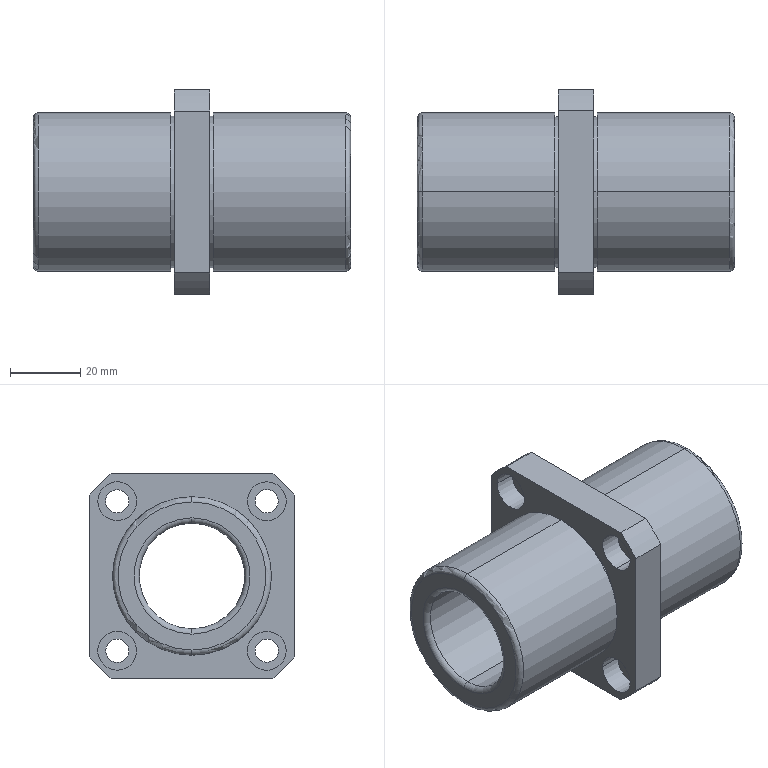Part | SolidWorks | features ICE 3, CirPattern 1, Fillet 1, Revolution 1 | 1 solid | 52 faces | box 90 x 58 x 58 mm | volume 93231 mm3 | cylinder 30 | plane 14 | torus 8 | commonest cylinder face diameters 6.6 x8 11 x8 43 x4 45 x4 74 x4 30 x2
STEP:
#1=CARTESIAN_POINT('',(-40.,0.,21.));
#2=VERTEX_POINT('',#1);
#3=CARTESIAN_POINT('',(-40.,0.,-21.));
#4=VERTEX_POINT('',#3);
#5=CARTESIAN_POINT('',(-40.,0.,0.));
#6=DIRECTION('',(-1.,0.,0.));
#7=DIRECTION('',(0.,0.,-1.));
#8=AXIS2_PLACEMENT_3D('',#5,#6,#7);
#9=CIRCLE('',#8,21.);
#10=EDGE_CURVE('',#2,#4,#9,.T.);
#11=ORIENTED_EDGE('',*,*,#10,.F.);
#12=CARTESIAN_POINT('',(-38.5,0.,22.5));
#13=VERTEX_POINT('',#12);
#14=CARTESIAN_POINT('',(-38.5,0.,21.));
#15=DIRECTION('',(0.,1.,0.));
#16=DIRECTION('',(0.,0.,1.));
#17=AXIS2_PLACEMENT_3D('',#14,#15,#16);
#18=CIRCLE('',#17,1.5);
#19=EDGE_CURVE('',#2,#13,#18,.T.);
#20=ORIENTED_EDGE('',*,*,#19,.T.);
#21=CARTESIAN_POINT('',(-38.5,0.,-22.5));
#22=VERTEX_POINT('',#21);
#23=CARTESIAN_POINT('',(-38.5,0.,0.));
#24=DIRECTION('',(1.,0.,0.));
#25=DIRECTION('',(0.,0.,-1.));
#26=AXIS2_PLACEMENT_3D('',#23,#24,#25);
#27=CIRCLE('',#26,22.5);
#28=EDGE_CURVE('',#22,#13,#27,.T.);
#29=ORIENTED_EDGE('',*,*,#28,.F.);
#30=CARTESIAN_POINT('',(-38.5,0.,-21.));
#31=DIRECTION('',(0.,-1.,0.));
#32=DIRECTION('',(0.,0.,-1.));
#33=AXIS2_PLACEMENT_3D('',#30,#31,#32);
#34=CIRCLE('',#33,1.5);
#35=EDGE_CURVE('',#4,#22,#34,.T.);
#36=ORIENTED_EDGE('',*,*,#35,.F.);
#37=EDGE_LOOP('',(#11,#20,#29,#36));
#38=FACE_OUTER_BOUND('',#37,.T.);
#39=CARTESIAN_POINT('',(-38.5,0.,0.));
#40=DIRECTION('',(1.,0.,0.));
#41=DIRECTION('',(0.,0.,-1.));
#42=AXIS2_PLACEMENT_3D('',#39,#40,#41);
#43=TOROIDAL_SURFACE('',#42,21.,1.5);
#44=ADVANCED_FACE('',(#38),#43,.T.);
#45=CARTESIAN_POINT('',(50.,0.,-21.));
#46=VERTEX_POINT('',#45);
#47=CARTESIAN_POINT('',(50.,0.,21.));
#48=VERTEX_POINT('',#47);
#49=CARTESIAN_POINT('',(50.,0.,0.));
#50=DIRECTION('',(1.,0.,0.));
#51=DIRECTION('',(0.,0.,1.));
#52=AXIS2_PLACEMENT_3D('',#49,#50,#51);
#53=CIRCLE('',#52,21.);
#54=EDGE_CURVE('',#46,#48,#53,.T.);
#55=ORIENTED_EDGE('',*,*,#54,.F.);
#56=CARTESIAN_POINT('',(48.5,0.,-22.5));
#57=VERTEX_POINT('',#56);
#58=CARTESIAN_POINT('',(48.5,0.,-21.));
#59=DIRECTION('',(0.,1.,0.));
#60=DIRECTION('',(0.,0.,1.));
#61=AXIS2_PLACEMENT_3D('',#58,#59,#60);
#62=CIRCLE('',#61,1.5);
#63=EDGE_CURVE('',#46,#57,#62,.T.);
#64=ORIENTED_EDGE('',*,*,#63,.T.);
#65=CARTESIAN_POINT('',(48.5,0.,22.5));
#66=VERTEX_POINT('',#65);
#67=CARTESIAN_POINT('',(48.5,0.,0.));
#68=DIRECTION('',(-1.,0.,0.));
#69=DIRECTION('',(0.,0.,1.));
#70=AXIS2_PLACEMENT_3D('',#67,#68,#69);
#71=CIRCLE('',#70,22.5);
#72=EDGE_CURVE('',#66,#57,#71,.T.);
#73=ORIENTED_EDGE('',*,*,#72,.F.);
#74=CARTESIAN_POINT('',(48.5,0.,21.));
#75=DIRECTION('',(0.,-1.,0.));
#76=DIRECTION('',(0.,0.,-1.));
#77=AXIS2_PLACEMENT_3D('',#74,#75,#76);
#78=CIRCLE('',#77,1.5);
#79=EDGE_CURVE('',#48,#66,#78,.T.);
#80=ORIENTED_EDGE('',*,*,#79,.F.);
#81=EDGE_LOOP('',(#55,#64,#73,#80));
#82=FACE_OUTER_BOUND('',#81,.T.);
#83=CARTESIAN_POINT('',(48.5,0.,0.));
#84=DIRECTION('',(-1.,0.,0.));
#85=DIRECTION('',(0.,0.,1.));
#86=AXIS2_PLACEMENT_3D('',#83,#84,#85);
#87=TOROIDAL_SURFACE('',#86,21.,1.5);
#88=ADVANCED_FACE('',(#82),#87,.T.);
#89=CARTESIAN_POINT('',(48.5,0.,-15.));
#90=VERTEX_POINT('',#89);
#91=CARTESIAN_POINT('',(48.5,0.,15.));
#92=VERTEX_POINT('',#91);
#93=CARTESIAN_POINT('',(48.5,0.,0.));
#94=DIRECTION('',(1.,0.,0.));
#95=DIRECTION('',(0.,0.,1.));
#96=AXIS2_PLACEMENT_3D('',#93,#94,#95);
#97=CIRCLE('',#96,15.);
#98=EDGE_CURVE('',#90,#92,#97,.T.);
#99=ORIENTED_EDGE('',*,*,#98,.F.);
#100=CARTESIAN_POINT('',(50.,0.,-16.5));
#101=VERTEX_POINT('',#100);
#102=CARTESIAN_POINT('',(48.5,0.,-16.5));
#103=DIRECTION('',(0.,1.,0.));
#104=DIRECTION('',(0.,0.,1.));
#105=AXIS2_PLACEMENT_3D('',#102,#103,#104);
#106=CIRCLE('',#105,1.5);
#107=EDGE_CURVE('',#90,#101,#106,.T.);
#108=ORIENTED_EDGE('',*,*,#107,.T.);
#109=CARTESIAN_POINT('',(50.,0.,16.5));
#110=VERTEX_POINT('',#109);
#111=CARTESIAN_POINT('',(50.,0.,0.));
#112=DIRECTION('',(-1.,0.,0.));
#113=DIRECTION('',(0.,0.,1.));
#114=AXIS2_PLACEMENT_3D('',#111,#112,#113);
#115=CIRCLE('',#114,16.5);
#116=EDGE_CURVE('',#110,#101,#115,.T.);
#117=ORIENTED_EDGE('',*,*,#116,.F.);
#118=CARTESIAN_POINT('',(48.5,0.,16.5));
#119=DIRECTION('',(0.,-1.,0.));
#120=DIRECTION('',(0.,0.,-1.));
#121=AXIS2_PLACEMENT_3D('',#118,#119,#120);
#122=CIRCLE('',#121,1.5);
#123=EDGE_CURVE('',#92,#110,#122,.T.);
#124=ORIENTED_EDGE('',*,*,#123,.F.);
#125=EDGE_LOOP('',(#99,#108,#117,#124));
#126=FACE_OUTER_BOUND('',#125,.T.);
#127=CARTESIAN_POINT('',(48.5,0.,0.));
#128=DIRECTION('',(-1.,0.,0.));
#129=DIRECTION('',(0.,0.,1.));
#130=AXIS2_PLACEMENT_3D('',#127,#128,#129);
#131=TOROIDAL_SURFACE('',#130,16.5,1.5);
#132=ADVANCED_FACE('',(#126),#131,.T.);
#133=CARTESIAN_POINT('',(-38.5,0.,15.));
#134=VERTEX_POINT('',#133);
#135=CARTESIAN_POINT('',(-38.5,0.,-15.));
#136=VERTEX_POINT('',#135);
#137=CARTESIAN_POINT('',(-38.5,0.,0.));
#138=DIRECTION('',(-1.,0.,0.));
#139=DIRECTION('',(0.,0.,-1.));
#140=AXIS2_PLACEMENT_3D('',#137,#138,#139);
#141=CIRCLE('',#140,15.);
#142=EDGE_CURVE('',#134,#136,#141,.T.);
#143=ORIENTED_EDGE('',*,*,#142,.F.);
#144=CARTESIAN_POINT('',(-40.,0.,16.5));
#145=VERTEX_POINT('',#144);
#146=CARTESIAN_POINT('',(-38.5,0.,16.5));
#147=DIRECTION('',(0.,1.,0.));
#148=DIRECTION('',(0.,0.,1.));
#149=AXIS2_PLACEMENT_3D('',#146,#147,#148);
#150=CIRCLE('',#149,1.5);
#151=EDGE_CURVE('',#134,#145,#150,.T.);
#152=ORIENTED_EDGE('',*,*,#151,.T.);
#153=CARTESIAN_POINT('',(-40.,0.,-16.5));
#154=VERTEX_POINT('',#153);
#155=CARTESIAN_POINT('',(-40.,0.,0.));
#156=DIRECTION('',(1.,0.,0.));
#157=DIRECTION('',(0.,0.,-1.));
#158=AXIS2_PLACEMENT_3D('',#155,#156,#157);
#159=CIRCLE('',#158,16.5);
#160=EDGE_CURVE('',#154,#145,#159,.T.);
#161=ORIENTED_EDGE('',*,*,#160,.F.);
#162=CARTESIAN_POINT('',(-38.5,0.,-16.5));
#163=DIRECTION('',(0.,-1.,0.));
#164=DIRECTION('',(0.,0.,-1.));
#165=AXIS2_PLACEMENT_3D('',#162,#163,#164);
#166=CIRCLE('',#165,1.5);
#167=EDGE_CURVE('',#136,#154,#166,.T.);
#168=ORIENTED_EDGE('',*,*,#167,.F.);
#169=EDGE_LOOP('',(#143,#152,#161,#168));
#170=FACE_OUTER_BOUND('',#169,.T.);
#171=CARTESIAN_POINT('',(-38.5,0.,0.));
#172=DIRECTION('',(1.,0.,0.));
#173=DIRECTION('',(0.,0.,-1.));
#174=AXIS2_PLACEMENT_3D('',#171,#172,#173);
#175=TOROIDAL_SURFACE('',#174,16.5,1.5);
#176=ADVANCED_FACE('',(#170),#175,.T.);
#177=CARTESIAN_POINT('',(10.,17.913,21.213));
#178=VERTEX_POINT('',#177);
#179=CARTESIAN_POINT('',(10.,24.513,21.213));
#180=VERTEX_POINT('',#179);
#181=CARTESIAN_POINT('',(10.,21.213,21.213));
#182=DIRECTION('',(1.,0.,0.));
#183=DIRECTION('',(0.,-1.,0.));
#184=AXIS2_PLACEMENT_3D('',#181,#182,#183);
#185=CIRCLE('',#184,3.3);
#186=EDGE_CURVE('',#178,#180,#185,.T.);
#187=ORIENTED_EDGE('',*,*,#186,.T.);
#188=CARTESIAN_POINT('',(6.1,24.513,21.213));
#189=VERTEX_POINT('',#188);
#190=CARTESIAN_POINT('',(50.001,24.513,21.213));
#191=DIRECTION('',(-1.,0.,0.));
#192=VECTOR('',#191,1000.);
#193=LINE('',#190,#192);
#194=EDGE_CURVE('',#180,#189,#193,.T.);
#195=ORIENTED_EDGE('',*,*,#194,.T.);
#196=CARTESIAN_POINT('',(6.1,17.913,21.213));
#197=VERTEX_POINT('',#196);
#198=CARTESIAN_POINT('',(6.1,21.213,21.213));
#199=DIRECTION('',(-1.,0.,0.));
#200=DIRECTION('',(0.,-1.,0.));
#201=AXIS2_PLACEMENT_3D('',#198,#199,#200);
#202=CIRCLE('',#201,3.3);
#203=EDGE_CURVE('',#189,#197,#202,.T.);
#204=ORIENTED_EDGE('',*,*,#203,.T.);
#205=CARTESIAN_POINT('',(50.001,17.913,21.213));
#206=DIRECTION('',(-1.,0.,0.));
#207=VECTOR('',#206,1000.);
#208=LINE('',#205,#207);
#209=EDGE_CURVE('',#178,#197,#208,.T.);
#210=ORIENTED_EDGE('',*,*,#209,.F.);
#211=EDGE_LOOP('',(#187,#195,#204,#210));
#212=FACE_OUTER_BOUND('',#211,.T.);
#213=CARTESIAN_POINT('',(50.001,21.213,21.213));
#214=DIRECTION('',(-1.,0.,0.));
#215=DIRECTION('',(0.,-1.,0.));
#216=AXIS2_PLACEMENT_3D('',#213,#214,#215);
#217=CYLINDRICAL_SURFACE('',#216,3.3);
#218=ADVANCED_FACE('',(#212),#217,.F.);
#219=CARTESIAN_POINT('',(6.1,26.713,21.213));
#220=VERTEX_POINT('',#219);
#221=CARTESIAN_POINT('',(6.1,15.713,21.213));
#222=VERTEX_POINT('',#221);
#223=CARTESIAN_POINT('',(6.1,21.213,21.213));
#224=DIRECTION('',(-1.,0.,0.));
#225=DIRECTION('',(0.,-1.,0.));
#226=AXIS2_PLACEMENT_3D('',#223,#224,#225);
#227=CIRCLE('',#226,5.5);
#228=EDGE_CURVE('',#220,#222,#227,.T.);
#229=ORIENTED_EDGE('',*,*,#228,.F.);
#230=CARTESIAN_POINT('',(0.,26.713,21.213));
#231=VERTEX_POINT('',#230);
#232=CARTESIAN_POINT('',(6.1,26.713,21.213));
#233=DIRECTION('',(-1.,0.,0.));
#234=VECTOR('',#233,1000.);
#235=LINE('',#232,#234);
#236=EDGE_CURVE('',#220,#231,#235,.T.);
#237=ORIENTED_EDGE('',*,*,#236,.T.);
#238=CARTESIAN_POINT('',(0.,15.713,21.213));
#239=VERTEX_POINT('',#238);
#240=CARTESIAN_POINT('',(0.,21.213,21.213));
#241=DIRECTION('',(-1.,0.,0.));
#242=DIRECTION('',(0.,-1.,0.));
#243=AXIS2_PLACEMENT_3D('',#240,#241,#242);
#244=CIRCLE('',#243,5.5);
#245=EDGE_CURVE('',#231,#239,#244,.T.);
#246=ORIENTED_EDGE('',*,*,#245,.T.);
#247=CARTESIAN_POINT('',(6.1,15.713,21.213));
#248=DIRECTION('',(-1.,0.,0.));
#249=VECTOR('',#248,1000.);
#250=LINE('',#247,#249);
#251=EDGE_CURVE('',#222,#239,#250,.T.);
#252=ORIENTED_EDGE('',*,*,#251,.F.);
#253=EDGE_LOOP('',(#229,#237,#246,#252));
#254=FACE_OUTER_BOUND('',#253,.T.);
#255=CARTESIAN_POINT('',(6.1,21.213,21.213));
#256=DIRECTION('',(-1.,0.,0.));
#257=DIRECTION('',(0.,-1.,0.));
#258=AXIS2_PLACEMENT_3D('',#255,#256,#257);
#259=CYLINDRICAL_SURFACE('',#258,5.5);
#260=ADVANCED_FACE('',(#254),#259,.F.);
#261=CARTESIAN_POINT('',(10.,-21.213,17.913));
#262=VERTEX_POINT('',#261);
#263=CARTESIAN_POINT('',(10.,-21.213,24.513));
#264=VERTEX_POINT('',#263);
#265=CARTESIAN_POINT('',(10.,-21.213,21.213));
#266=DIRECTION('',(1.,0.,0.));
#267=DIRECTION('',(0.,0.,-1.));
#268=AXIS2_PLACEMENT_3D('',#265,#266,#267);
#269=CIRCLE('',#268,3.3);
#270=EDGE_CURVE('',#262,#264,#269,.T.);
#271=ORIENTED_EDGE('',*,*,#270,.T.);
#272=CARTESIAN_POINT('',(6.1,-21.213,24.513));
#273=VERTEX_POINT('',#272);
#274=CARTESIAN_POINT('',(50.001,-21.213,24.513));
#275=DIRECTION('',(-1.,0.,0.));
#276=VECTOR('',#275,1000.);
#277=LINE('',#274,#276);
#278=EDGE_CURVE('',#264,#273,#277,.T.);
#279=ORIENTED_EDGE('',*,*,#278,.T.);
#280=CARTESIAN_POINT('',(6.1,-21.213,17.913));
#281=VERTEX_POINT('',#280);
#282=CARTESIAN_POINT('',(6.1,-21.213,21.213));
#283=DIRECTION('',(-1.,0.,0.));
#284=DIRECTION('',(0.,0.,-1.));
#285=AXIS2_PLACEMENT_3D('',#282,#283,#284);
#286=CIRCLE('',#285,3.3);
#287=EDGE_CURVE('',#273,#281,#286,.T.);
#288=ORIENTED_EDGE('',*,*,#287,.T.);
#289=CARTESIAN_POINT('',(50.001,-21.213,17.913));
#290=DIRECTION('',(-1.,0.,0.));
#291=VECTOR('',#290,1000.);
#292=LINE('',#289,#291);
#293=EDGE_CURVE('',#262,#281,#292,.T.);
#294=ORIENTED_EDGE('',*,*,#293,.F.);
#295=EDGE_LOOP('',(#271,#279,#288,#294));
#296=FACE_OUTER_BOUND('',#295,.T.);
#297=CARTESIAN_POINT('',(50.001,-21.213,21.213));
#298=DIRECTION('',(-1.,0.,0.));
#299=DIRECTION('',(0.,0.,-1.));
#300=AXIS2_PLACEMENT_3D('',#297,#298,#299);
#301=CYLINDRICAL_SURFACE('',#300,3.3);
#302=ADVANCED_FACE('',(#296),#301,.F.);
#303=CARTESIAN_POINT('',(6.1,-21.213,26.713));
#304=VERTEX_POINT('',#303);
#305=CARTESIAN_POINT('',(6.1,-21.213,15.713));
#306=VERTEX_POINT('',#305);
#307=CARTESIAN_POINT('',(6.1,-21.213,21.213));
#308=DIRECTION('',(-1.,0.,0.));
#309=DIRECTION('',(0.,0.,-1.));
#310=AXIS2_PLACEMENT_3D('',#307,#308,#309);
#311=CIRCLE('',#310,5.5);
#312=EDGE_CURVE('',#304,#306,#311,.T.);
#313=ORIENTED_EDGE('',*,*,#312,.F.);
#314=CARTESIAN_POINT('',(0.,-21.213,26.713));
#315=VERTEX_POINT('',#314);
#316=CARTESIAN_POINT('',(6.1,-21.213,26.713));
#317=DIRECTION('',(-1.,0.,0.));
#318=VECTOR('',#317,1000.);
#319=LINE('',#316,#318);
#320=EDGE_CURVE('',#304,#315,#319,.T.);
#321=ORIENTED_EDGE('',*,*,#320,.T.);
#322=CARTESIAN_POINT('',(0.,-21.213,15.713));
#323=VERTEX_POINT('',#322);
#324=CARTESIAN_POINT('',(0.,-21.213,21.213));
#325=DIRECTION('',(-1.,0.,0.));
#326=DIRECTION('',(0.,0.,-1.));
#327=AXIS2_PLACEMENT_3D('',#324,#325,#326);
#328=CIRCLE('',#327,5.5);
#329=EDGE_CURVE('',#315,#323,#328,.T.);
#330=ORIENTED_EDGE('',*,*,#329,.T.);
#331=CARTESIAN_POINT('',(6.1,-21.213,15.713));
#332=DIRECTION('',(-1.,0.,0.));
#333=VECTOR('',#332,1000.);
#334=LINE('',#331,#333);
#335=EDGE_CURVE('',#306,#323,#334,.T.);
#336=ORIENTED_EDGE('',*,*,#335,.F.);
#337=EDGE_LOOP('',(#313,#321,#330,#336));
#338=FACE_OUTER_BOUND('',#337,.T.);
#339=CARTESIAN_POINT('',(6.1,-21.213,21.213));
#340=DIRECTION('',(-1.,0.,0.));
#341=DIRECTION('',(0.,0.,-1.));
#342=AXIS2_PLACEMENT_3D('',#339,#340,#341);
#343=CYLINDRICAL_SURFACE('',#342,5.5);
#344=ADVANCED_FACE('',(#338),#343,.F.);
#345=CARTESIAN_POINT('',(10.,-17.913,-21.213));
#346=VERTEX_POINT('',#345);
#347=CARTESIAN_POINT('',(10.,-24.513,-21.213));
#348=VERTEX_POINT('',#347);
#349=CARTESIAN_POINT('',(10.,-21.213,-21.213));
#350=DIRECTION('',(1.,0.,0.));
#351=DIRECTION('',(0.,1.,0.));
#352=AXIS2_PLACEMENT_3D('',#349,#350,#351);
#353=CIRCLE('',#352,3.3);
#354=EDGE_CURVE('',#346,#348,#353,.T.);
#355=ORIENTED_EDGE('',*,*,#354,.T.);
#356=CARTESIAN_POINT('',(6.1,-24.513,-21.213));
#357=VERTEX_POINT('',#356);
#358=CARTESIAN_POINT('',(50.001,-24.513,-21.213));
#359=DIRECTION('',(-1.,0.,0.));
#360=VECTOR('',#359,1000.);
#361=LINE('',#358,#360);
#362=EDGE_CURVE('',#348,#357,#361,.T.);
#363=ORIENTED_EDGE('',*,*,#362,.T.);
#364=CARTESIAN_POINT('',(6.1,-17.913,-21.213));
#365=VERTEX_POINT('',#364);
#366=CARTESIAN_POINT('',(6.1,-21.213,-21.213));
#367=DIRECTION('',(-1.,0.,0.));
#368=DIRECTION('',(0.,1.,0.));
#369=AXIS2_PLACEMENT_3D('',#366,#367,#368);
#370=CIRCLE('',#369,3.3);
#371=EDGE_CURVE('',#357,#365,#370,.T.);
#372=ORIENTED_EDGE('',*,*,#371,.T.);
#373=CARTESIAN_POINT('',(50.001,-17.913,-21.213));
#374=DIRECTION('',(-1.,0.,0.));
#375=VECTOR('',#374,1000.);
#376=LINE('',#373,#375);
#377=EDGE_CURVE('',#346,#365,#376,.T.);
#378=ORIENTED_EDGE('',*,*,#377,.F.);
#379=EDGE_LOOP('',(#355,#363,#372,#378));
#380=FACE_OUTER_BOUND('',#379,.T.);
#381=CARTESIAN_POINT('',(50.001,-21.213,-21.213));
#382=DIRECTION('',(-1.,0.,0.));
#383=DIRECTION('',(0.,1.,0.));
#384=AXIS2_PLACEMENT_3D('',#381,#382,#383);
#385=CYLINDRICAL_SURFACE('',#384,3.3);
#386=ADVANCED_FACE('',(#380),#385,.F.);
#387=CARTESIAN_POINT('',(6.1,-26.713,-21.213));
#388=VERTEX_POINT('',#387);
#389=CARTESIAN_POINT('',(6.1,-15.713,-21.213));
#390=VERTEX_POINT('',#389);
#391=CARTESIAN_POINT('',(6.1,-21.213,-21.213));
#392=DIRECTION('',(-1.,0.,0.));
#393=DIRECTION('',(0.,1.,0.));
#394=AXIS2_PLACEMENT_3D('',#391,#392,#393);
#395=CIRCLE('',#394,5.5);
#396=EDGE_CURVE('',#388,#390,#395,.T.);
#397=ORIENTED_EDGE('',*,*,#396,.F.);
#398=CARTESIAN_POINT('',(0.,-26.713,-21.213));
#399=VERTEX_POINT('',#398);
#400=CARTESIAN_POINT('',(6.1,-26.713,-21.213));
#401=DIRECTION('',(-1.,0.,0.));
#402=VECTOR('',#401,1000.);
#403=LINE('',#400,#402);
#404=EDGE_CURVE('',#388,#399,#403,.T.);
#405=ORIENTED_EDGE('',*,*,#404,.T.);
#406=CARTESIAN_POINT('',(0.,-15.713,-21.213));
#407=VERTEX_POINT('',#406);
#408=CARTESIAN_POINT('',(0.,-21.213,-21.213));
#409=DIRECTION('',(-1.,0.,0.));
#410=DIRECTION('',(0.,1.,0.));
#411=AXIS2_PLACEMENT_3D('',#408,#409,#410);
#412=CIRCLE('',#411,5.5);
#413=EDGE_CURVE('',#399,#407,#412,.T.);
#414=ORIENTED_EDGE('',*,*,#413,.T.);
#415=CARTESIAN_POINT('',(6.1,-15.713,-21.213));
#416=DIRECTION('',(-1.,0.,0.));
#417=VECTOR('',#416,1000.);
#418=LINE('',#415,#417);
#419=EDGE_CURVE('',#390,#407,#418,.T.);
#420=ORIENTED_EDGE('',*,*,#419,.F.);
#421=EDGE_LOOP('',(#397,#405,#414,#420));
#422=FACE_OUTER_BOUND('',#421,.T.);
#423=CARTESIAN_POINT('',(6.1,-21.213,-21.213));
#424=DIRECTION('',(-1.,0.,0.));
#425=DIRECTION('',(0.,1.,0.));
#426=AXIS2_PLACEMENT_3D('',#423,#424,#425);
#427=CYLINDRICAL_SURFACE('',#426,5.5);
#428=ADVANCED_FACE('',(#422),#427,.F.);
#429=CARTESIAN_POINT('',(10.,21.213,-17.913));
#430=VERTEX_POINT('',#429);
#431=CARTESIAN_POINT('',(10.,21.213,-24.513));
#432=VERTEX_POINT('',#431);
#433=CARTESIAN_POINT('',(10.,21.213,-21.213));
#434=DIRECTION('',(1.,0.,0.));
#435=DIRECTION('',(0.,0.,1.));
#436=AXIS2_PLACEMENT_3D('',#433,#434,#435);
#437=CIRCLE('',#436,3.3);
#438=EDGE_CURVE('',#430,#432,#437,.T.);
#439=ORIENTED_EDGE('',*,*,#438,.T.);
#440=CARTESIAN_POINT('',(6.1,21.213,-24.513));
#441=VERTEX_POINT('',#440);
#442=CARTESIAN_POINT('',(50.001,21.213,-24.513));
#443=DIRECTION('',(-1.,0.,0.));
#444=VECTOR('',#443,1000.);
#445=LINE('',#442,#444);
#446=EDGE_CURVE('',#432,#441,#445,.T.);
#447=ORIENTED_EDGE('',*,*,#446,.T.);
#448=CARTESIAN_POINT('',(6.1,21.213,-17.913));
#449=VERTEX_POINT('',#448);
#450=CARTESIAN_POINT('',(6.1,21.213,-21.213));
#451=DIRECTION('',(-1.,0.,0.));
#452=DIRECTION('',(0.,0.,1.));
#453=AXIS2_PLACEMENT_3D('',#450,#451,#452);
#454=CIRCLE('',#453,3.3);
#455=EDGE_CURVE('',#441,#449,#454,.T.);
#456=ORIENTED_EDGE('',*,*,#455,.T.);
#457=CARTESIAN_POINT('',(50.001,21.213,-17.913));
#458=DIRECTION('',(-1.,0.,0.));
#459=VECTOR('',#458,1000.);
#460=LINE('',#457,#459);
#461=EDGE_CURVE('',#430,#449,#460,.T.);
#462=ORIENTED_EDGE('',*,*,#461,.F.);
#463=EDGE_LOOP('',(#439,#447,#456,#462));
#464=FACE_OUTER_BOUND('',#463,.T.);
#465=CARTESIAN_POINT('',(50.001,21.213,-21.213));
#466=DIRECTION('',(-1.,0.,0.));
#467=DIRECTION('',(0.,0.,1.));
#468=AXIS2_PLACEMENT_3D('',#465,#466,#467);
#469=CYLINDRICAL_SURFACE('',#468,3.3);
#470=ADVANCED_FACE('',(#464),#469,.F.);
#471=CARTESIAN_POINT('',(6.1,21.213,-26.713));
#472=VERTEX_POINT('',#471);
#473=CARTESIAN_POINT('',(6.1,21.213,-15.713));
#474=VERTEX_POINT('',#473);
#475=CARTESIAN_POINT('',(6.1,21.213,-21.213));
#476=DIRECTION('',(-1.,0.,0.));
#477=DIRECTION('',(0.,0.,1.));
#478=AXIS2_PLACEMENT_3D('',#475,#476,#477);
#479=CIRCLE('',#478,5.5);
#480=EDGE_CURVE('',#472,#474,#479,.T.);
#481=ORIENTED_EDGE('',*,*,#480,.F.);
#482=CARTESIAN_POINT('',(0.,21.213,-26.713));
#483=VERTEX_POINT('',#482);
#484=CARTESIAN_POINT('',(6.1,21.213,-26.713));
#485=DIRECTION('',(-1.,0.,0.));
#486=VECTOR('',#485,1000.);
#487=LINE('',#484,#486);
#488=EDGE_CURVE('',#472,#483,#487,.T.);
#489=ORIENTED_EDGE('',*,*,#488,.T.);
#490=CARTESIAN_POINT('',(0.,21.213,-15.713));
#491=VERTEX_POINT('',#490);
#492=CARTESIAN_POINT('',(0.,21.213,-21.213));
#493=DIRECTION('',(-1.,0.,0.));
#494=DIRECTION('',(0.,0.,1.));
#495=AXIS2_PLACEMENT_3D('',#492,#493,#494);
#496=CIRCLE('',#495,5.5);
#497=EDGE_CURVE('',#483,#491,#496,.T.);
#498=ORIENTED_EDGE('',*,*,#497,.T.);
#499=CARTESIAN_POINT('',(6.1,21.213,-15.713));
#500=DIRECTION('',(-1.,0.,0.));
#501=VECTOR('',#500,1000.);
#502=LINE('',#499,#501);
#503=EDGE_CURVE('',#474,#491,#502,.T.);
#504=ORIENTED_EDGE('',*,*,#503,.F.);
#505=EDGE_LOOP('',(#481,#489,#498,#504));
#506=FACE_OUTER_BOUND('',#505,.T.);
#507=CARTESIAN_POINT('',(6.1,21.213,-21.213));
#508=DIRECTION('',(-1.,0.,0.));
#509=DIRECTION('',(0.,0.,1.));
#510=AXIS2_PLACEMENT_3D('',#507,#508,#509);
#511=CYLINDRICAL_SURFACE('',#510,5.5);
#512=ADVANCED_FACE('',(#506),#511,.F.);
#513=CARTESIAN_POINT('',(11.,0.,21.5));
#514=VERTEX_POINT('',#513);
#515=CARTESIAN_POINT('',(11.,0.,-21.5));
#516=VERTEX_POINT('',#515);
#517=CARTESIAN_POINT('',(11.,0.,0.));
#518=DIRECTION('',(-1.,0.,0.));
#519=DIRECTION('',(0.,0.,1.));
#520=AXIS2_PLACEMENT_3D('',#517,#518,#519);
#521=CIRCLE('',#520,21.5);
#522=EDGE_CURVE('',#514,#516,#521,.T.);
#523=ORIENTED_EDGE('',*,*,#522,.T.);
#524=CARTESIAN_POINT('',(10.,0.,-21.5));
#525=VERTEX_POINT('',#524);
#526=CARTESIAN_POINT('',(64.,0.,-21.5));
#527=DIRECTION('',(-1.,0.,0.));
#528=VECTOR('',#527,1000.);
#529=LINE('',#526,#528);
#530=EDGE_CURVE('',#516,#525,#529,.T.);
#531=ORIENTED_EDGE('',*,*,#530,.T.);
#532=CARTESIAN_POINT('',(10.,0.,21.5));
#533=VERTEX_POINT('',#532);
#534=CARTESIAN_POINT('',(10.,0.,0.));
#535=DIRECTION('',(-1.,0.,0.));
#536=DIRECTION('',(0.,0.,1.));
#537=AXIS2_PLACEMENT_3D('',#534,#535,#536);
#538=CIRCLE('',#537,21.5);
#539=EDGE_CURVE('',#533,#525,#538,.T.);
#540=ORIENTED_EDGE('',*,*,#539,.F.);
#541=CARTESIAN_POINT('',(64.,0.,21.5));
#542=DIRECTION('',(-1.,0.,0.));
#543=VECTOR('',#542,1000.);
#544=LINE('',#541,#543);
#545=EDGE_CURVE('',#514,#533,#544,.T.);
#546=ORIENTED_EDGE('',*,*,#545,.F.);
#547=EDGE_LOOP('',(#523,#531,#540,#546));
#548=FACE_OUTER_BOUND('',#547,.T.);
#549=CARTESIAN_POINT('',(64.,0.,0.));
#550=DIRECTION('',(-1.,0.,0.));
#551=DIRECTION('',(0.,0.,1.));
#552=AXIS2_PLACEMENT_3D('',#549,#550,#551);
#553=CYLINDRICAL_SURFACE('',#552,21.5);
#554=ADVANCED_FACE('',(#548),#553,.T.);
#555=ORIENTED_EDGE('',*,*,#72,.T.);
#556=CARTESIAN_POINT('',(11.,0.,-22.5));
#557=VERTEX_POINT('',#556);
#558=CARTESIAN_POINT('',(64.,0.,-22.5));
#559=DIRECTION('',(-1.,0.,0.));
#560=VECTOR('',#559,1000.);
#561=LINE('',#558,#560);
#562=EDGE_CURVE('',#57,#557,#561,.T.);
#563=ORIENTED_EDGE('',*,*,#562,.T.);
#564=CARTESIAN_POINT('',(11.,0.,22.5));
#565=VERTEX_POINT('',#564);
#566=CARTESIAN_POINT('',(11.,0.,0.));
#567=DIRECTION('',(-1.,0.,0.));
#568=DIRECTION('',(0.,0.,1.));
#569=AXIS2_PLACEMENT_3D('',#566,#567,#568);
#570=CIRCLE('',#569,22.5);
#571=EDGE_CURVE('',#565,#557,#570,.T.);
#572=ORIENTED_EDGE('',*,*,#571,.F.);
#573=CARTESIAN_POINT('',(64.,0.,22.5));
#574=DIRECTION('',(-1.,0.,0.));
#575=VECTOR('',#574,1000.);
#576=LINE('',#573,#575);
#577=EDGE_CURVE('',#66,#565,#576,.T.);
#578=ORIENTED_EDGE('',*,*,#577,.F.);
#579=EDGE_LOOP('',(#555,#563,#572,#578));
#580=FACE_OUTER_BOUND('',#579,.T.);
#581=CARTESIAN_POINT('',(64.,0.,0.));
#582=DIRECTION('',(-1.,0.,0.));
#583=DIRECTION('',(0.,0.,1.));
#584=AXIS2_PLACEMENT_3D('',#581,#582,#583);
#585=CYLINDRICAL_SURFACE('',#584,22.5);
#586=ADVANCED_FACE('',(#580),#585,.T.);
#587=CARTESIAN_POINT('',(48.5,0.,0.));
#588=DIRECTION('',(1.,0.,0.));
#589=DIRECTION('',(0.,0.,1.));
#590=AXIS2_PLACEMENT_3D('',#587,#588,#589);
#591=CIRCLE('',#590,15.);
#592=EDGE_CURVE('',#92,#90,#591,.T.);
#593=ORIENTED_EDGE('',*,*,#592,.T.);
#594=CARTESIAN_POINT('',(64.,0.,-15.));
#595=DIRECTION('',(-1.,0.,0.));
#596=VECTOR('',#595,1000.);
#597=LINE('',#594,#596);
#598=EDGE_CURVE('',#90,#136,#597,.T.);
#599=ORIENTED_EDGE('',*,*,#598,.T.);
#600=CARTESIAN_POINT('',(-38.5,0.,0.));
#601=DIRECTION('',(-1.,0.,0.));
#602=DIRECTION('',(0.,0.,-1.));
#603=AXIS2_PLACEMENT_3D('',#600,#601,#602);
#604=CIRCLE('',#603,15.);
#605=EDGE_CURVE('',#136,#134,#604,.T.);
#606=ORIENTED_EDGE('',*,*,#605,.T.);
#607=CARTESIAN_POINT('',(64.,0.,15.));
#608=DIRECTION('',(-1.,0.,0.));
#609=VECTOR('',#608,1000.);
#610=LINE('',#607,#609);
#611=EDGE_CURVE('',#92,#134,#610,.T.);
#612=ORIENTED_EDGE('',*,*,#611,.F.);
#613=EDGE_LOOP('',(#593,#599,#606,#612));
#614=FACE_OUTER_BOUND('',#613,.T.);
#615=CARTESIAN_POINT('',(64.,0.,0.));
#616=DIRECTION('',(-1.,0.,0.));
#617=DIRECTION('',(0.,0.,1.));
#618=AXIS2_PLACEMENT_3D('',#615,#616,#617);
#619=CYLINDRICAL_SURFACE('',#618,15.);
#620=ADVANCED_FACE('',(#614),#619,.F.);
#621=CARTESIAN_POINT('',(-1.,0.,22.5));
#622=VERTEX_POINT('',#621);
#623=CARTESIAN_POINT('',(-1.,0.,-22.5));
#624=VERTEX_POINT('',#623);
#625=CARTESIAN_POINT('',(-1.,0.,0.));
#626=DIRECTION('',(-1.,0.,0.));
#627=DIRECTION('',(0.,0.,1.));
#628=AXIS2_PLACEMENT_3D('',#625,#626,#627);
#629=CIRCLE('',#628,22.5);
#630=EDGE_CURVE('',#622,#624,#629,.T.);
#631=ORIENTED_EDGE('',*,*,#630,.T.);
#632=CARTESIAN_POINT('',(64.,0.,-22.5));
#633=DIRECTION('',(-1.,0.,0.));
#634=VECTOR('',#633,1000.);
#635=LINE('',#632,#634);
#636=EDGE_CURVE('',#624,#22,#635,.T.);
#637=ORIENTED_EDGE('',*,*,#636,.T.);
#638=ORIENTED_EDGE('',*,*,#28,.T.);
#639=CARTESIAN_POINT('',(64.,0.,22.5));
#640=DIRECTION('',(-1.,0.,0.));
#641=VECTOR('',#640,1000.);
#642=LINE('',#639,#641);
#643=EDGE_CURVE('',#622,#13,#642,.T.);
#644=ORIENTED_EDGE('',*,*,#643,.F.);
#645=EDGE_LOOP('',(#631,#637,#638,#644));
#646=FACE_OUTER_BOUND('',#645,.T.);
#647=CARTESIAN_POINT('',(64.,0.,0.));
#648=DIRECTION('',(-1.,0.,0.));
#649=DIRECTION('',(0.,0.,1.));
#650=AXIS2_PLACEMENT_3D('',#647,#648,#649);
#651=CYLINDRICAL_SURFACE('',#650,22.5);
#652=ADVANCED_FACE('',(#646),#651,.T.);
#653=CARTESIAN_POINT('',(0.,0.,21.5));
#654=VERTEX_POINT('',#653);
#655=CARTESIAN_POINT('',(0.,0.,-21.5));
#656=VERTEX_POINT('',#655);
#657=CARTESIAN_POINT('',(0.,0.,0.));
#658=DIRECTION('',(-1.,0.,0.));
#659=DIRECTION('',(0.,0.,1.));
#660=AXIS2_PLACEMENT_3D('',#657,#658,#659);
#661=CIRCLE('',#660,21.5);
#662=EDGE_CURVE('',#654,#656,#661,.T.);
#663=ORIENTED_EDGE('',*,*,#662,.T.);
#664=CARTESIAN_POINT('',(-1.,0.,-21.5));
#665=VERTEX_POINT('',#664);
#666=CARTESIAN_POINT('',(64.,0.,-21.5));
#667=DIRECTION('',(-1.,0.,0.));
#668=VECTOR('',#667,1000.);
#669=LINE('',#666,#668);
#670=EDGE_CURVE('',#656,#665,#669,.T.);
#671=ORIENTED_EDGE('',*,*,#670,.T.);
#672=CARTESIAN_POINT('',(-1.,0.,21.5));
#673=VERTEX_POINT('',#672);
#674=CARTESIAN_POINT('',(-1.,0.,0.));
#675=DIRECTION('',(-1.,0.,0.));
#676=DIRECTION('',(0.,0.,1.));
#677=AXIS2_PLACEMENT_3D('',#674,#675,#676);
#678=CIRCLE('',#677,21.5);
#679=EDGE_CURVE('',#673,#665,#678,.T.);
#680=ORIENTED_EDGE('',*,*,#679,.F.);
#681=CARTESIAN_POINT('',(64.,0.,21.5));
#682=DIRECTION('',(-1.,0.,0.));
#683=VECTOR('',#682,1000.);
#684=LINE('',#681,#683);
#685=EDGE_CURVE('',#654,#673,#684,.T.);
#686=ORIENTED_EDGE('',*,*,#685,.F.);
#687=EDGE_LOOP('',(#663,#671,#680,#686));
#688=FACE_OUTER_BOUND('',#687,.T.);
#689=CARTESIAN_POINT('',(64.,0.,0.));
#690=DIRECTION('',(-1.,0.,0.));
#691=DIRECTION('',(0.,0.,1.));
#692=AXIS2_PLACEMENT_3D('',#689,#690,#691);
#693=CYLINDRICAL_SURFACE('',#692,21.5);
#694=ADVANCED_FACE('',(#688),#693,.T.);
#695=CARTESIAN_POINT('',(10.,-29.,22.978));
#696=VERTEX_POINT('',#695);
#697=CARTESIAN_POINT('',(10.,-22.978,29.));
#698=VERTEX_POINT('',#697);
#699=CARTESIAN_POINT('',(10.,0.,0.));
#700=DIRECTION('',(-1.,0.,0.));
#701=DIRECTION('',(0.,0.,1.));
#702=AXIS2_PLACEMENT_3D('',#699,#700,#701);
#703=CIRCLE('',#702,37.);
#704=EDGE_CURVE('',#696,#698,#703,.T.);
#705=ORIENTED_EDGE('',*,*,#704,.T.);
#706=CARTESIAN_POINT('',(0.,-22.978,29.));
#707=VERTEX_POINT('',#706);
#708=CARTESIAN_POINT('',(64.,-22.978,29.));
#709=DIRECTION('',(-1.,0.,0.));
#710=VECTOR('',#709,1000.);
#711=LINE('',#708,#710);
#712=EDGE_CURVE('',#698,#707,#711,.T.);
#713=ORIENTED_EDGE('',*,*,#712,.T.);
#714=CARTESIAN_POINT('',(0.,-29.,22.978));
#715=VERTEX_POINT('',#714);
#716=CARTESIAN_POINT('',(0.,0.,0.));
#717=DIRECTION('',(-1.,0.,0.));
#718=DIRECTION('',(0.,0.,1.));
#719=AXIS2_PLACEMENT_3D('',#716,#717,#718);
#720=CIRCLE('',#719,37.);
#721=EDGE_CURVE('',#715,#707,#720,.T.);
#722=ORIENTED_EDGE('',*,*,#721,.F.);
#723=CARTESIAN_POINT('',(64.,-29.,22.978));
#724=DIRECTION('',(1.,0.,0.));
#725=VECTOR('',#724,1000.);
#726=LINE('',#723,#725);
#727=EDGE_CURVE('',#715,#696,#726,.T.);
#728=ORIENTED_EDGE('',*,*,#727,.T.);
#729=EDGE_LOOP('',(#705,#713,#722,#728));
#730=FACE_OUTER_BOUND('',#729,.T.);
#731=CARTESIAN_POINT('',(64.,0.,0.));
#732=DIRECTION('',(-1.,0.,0.));
#733=DIRECTION('',(0.,0.,1.));
#734=AXIS2_PLACEMENT_3D('',#731,#732,#733);
#735=CYLINDRICAL_SURFACE('',#734,37.);
#736=ADVANCED_FACE('',(#730),#735,.T.);
#737=CARTESIAN_POINT('',(10.,-22.978,-29.));
#738=VERTEX_POINT('',#737);
#739=CARTESIAN_POINT('',(10.,-29.,-22.978));
#740=VERTEX_POINT('',#739);
#741=CARTESIAN_POINT('',(10.,0.,0.));
#742=DIRECTION('',(-1.,0.,0.));
#743=DIRECTION('',(0.,0.,1.));
#744=AXIS2_PLACEMENT_3D('',#741,#742,#743);
#745=CIRCLE('',#744,37.);
#746=EDGE_CURVE('',#738,#740,#745,.T.);
#747=ORIENTED_EDGE('',*,*,#746,.T.);
#748=CARTESIAN_POINT('',(0.,-29.,-22.978));
#749=VERTEX_POINT('',#748);
#750=CARTESIAN_POINT('',(64.,-29.,-22.978));
#751=DIRECTION('',(-1.,0.,0.));
#752=VECTOR('',#751,1000.);
#753=LINE('',#750,#752);
#754=EDGE_CURVE('',#740,#749,#753,.T.);
#755=ORIENTED_EDGE('',*,*,#754,.T.);
#756=CARTESIAN_POINT('',(0.,-22.978,-29.));
#757=VERTEX_POINT('',#756);
#758=CARTESIAN_POINT('',(0.,0.,0.));
#759=DIRECTION('',(-1.,0.,0.));
#760=DIRECTION('',(0.,0.,1.));
#761=AXIS2_PLACEMENT_3D('',#758,#759,#760);
#762=CIRCLE('',#761,37.);
#763=EDGE_CURVE('',#757,#749,#762,.T.);
#764=ORIENTED_EDGE('',*,*,#763,.F.);
#765=CARTESIAN_POINT('',(64.,-22.978,-29.));
#766=DIRECTION('',(1.,0.,0.));
#767=VECTOR('',#766,1000.);
#768=LINE('',#765,#767);
#769=EDGE_CURVE('',#757,#738,#768,.T.);
#770=ORIENTED_EDGE('',*,*,#769,.T.);
#771=EDGE_LOOP('',(#747,#755,#764,#770));
#772=FACE_OUTER_BOUND('',#771,.T.);
#773=CARTESIAN_POINT('',(64.,0.,0.));
#774=DIRECTION('',(-1.,0.,0.));
#775=DIRECTION('',(0.,0.,1.));
#776=AXIS2_PLACEMENT_3D('',#773,#774,#775);
#777=CYLINDRICAL_SURFACE('',#776,37.);
#778=ADVANCED_FACE('',(#772),#777,.T.);
#779=CARTESIAN_POINT('',(10.,29.,-22.978));
#780=VERTEX_POINT('',#779);
#781=CARTESIAN_POINT('',(10.,22.978,-29.));
#782=VERTEX_POINT('',#781);
#783=CARTESIAN_POINT('',(10.,0.,0.));
#784=DIRECTION('',(-1.,0.,0.));
#785=DIRECTION('',(0.,0.,1.));
#786=AXIS2_PLACEMENT_3D('',#783,#784,#785);
#787=CIRCLE('',#786,37.);
#788=EDGE_CURVE('',#780,#782,#787,.T.);
#789=ORIENTED_EDGE('',*,*,#788,.T.);
#790=CARTESIAN_POINT('',(0.,22.978,-29.));
#791=VERTEX_POINT('',#790);
#792=CARTESIAN_POINT('',(64.,22.978,-29.));
#793=DIRECTION('',(-1.,0.,0.));
#794=VECTOR('',#793,1000.);
#795=LINE('',#792,#794);
#796=EDGE_CURVE('',#782,#791,#795,.T.);
#797=ORIENTED_EDGE('',*,*,#796,.T.);
#798=CARTESIAN_POINT('',(0.,29.,-22.978));
#799=VERTEX_POINT('',#798);
#800=CARTESIAN_POINT('',(0.,0.,0.));
#801=DIRECTION('',(-1.,0.,0.));
#802=DIRECTION('',(0.,0.,1.));
#803=AXIS2_PLACEMENT_3D('',#800,#801,#802);
#804=CIRCLE('',#803,37.);
#805=EDGE_CURVE('',#799,#791,#804,.T.);
#806=ORIENTED_EDGE('',*,*,#805,.F.);
#807=CARTESIAN_POINT('',(64.,29.,-22.978));
#808=DIRECTION('',(1.,0.,0.));
#809=VECTOR('',#808,1000.);
#810=LINE('',#807,#809);
#811=EDGE_CURVE('',#799,#780,#810,.T.);
#812=ORIENTED_EDGE('',*,*,#811,.T.);
#813=EDGE_LOOP('',(#789,#797,#806,#812));
#814=FACE_OUTER_BOUND('',#813,.T.);
#815=CARTESIAN_POINT('',(64.,0.,0.));
#816=DIRECTION('',(-1.,0.,0.));
#817=DIRECTION('',(0.,0.,1.));
#818=AXIS2_PLACEMENT_3D('',#815,#816,#817);
#819=CYLINDRICAL_SURFACE('',#818,37.);
#820=ADVANCED_FACE('',(#814),#819,.T.);
#821=CARTESIAN_POINT('',(0.,22.978,29.));
#822=VERTEX_POINT('',#821);
#823=CARTESIAN_POINT('',(0.,29.,22.978));
#824=VERTEX_POINT('',#823);
#825=CARTESIAN_POINT('',(0.,0.,0.));
#826=DIRECTION('',(-1.,0.,0.));
#827=DIRECTION('',(0.,0.,1.));
#828=AXIS2_PLACEMENT_3D('',#825,#826,#827);
#829=CIRCLE('',#828,37.);
#830=EDGE_CURVE('',#822,#824,#829,.T.);
#831=ORIENTED_EDGE('',*,*,#830,.F.);
#832=CARTESIAN_POINT('',(10.,22.978,29.));
#833=VERTEX_POINT('',#832);
#834=CARTESIAN_POINT('',(64.,22.978,29.));
#835=DIRECTION('',(1.,0.,0.));
#836=VECTOR('',#835,1000.);
#837=LINE('',#834,#836);
#838=EDGE_CURVE('',#822,#833,#837,.T.);
#839=ORIENTED_EDGE('',*,*,#838,.T.);
#840=CARTESIAN_POINT('',(10.,29.,22.978));
#841=VERTEX_POINT('',#840);
#842=CARTESIAN_POINT('',(10.,0.,0.));
#843=DIRECTION('',(-1.,0.,0.));
#844=DIRECTION('',(0.,0.,1.));
#845=AXIS2_PLACEMENT_3D('',#842,#843,#844);
#846=CIRCLE('',#845,37.);
#847=EDGE_CURVE('',#833,#841,#846,.T.);
#848=ORIENTED_EDGE('',*,*,#847,.T.);
#849=CARTESIAN_POINT('',(64.,29.,22.978));
#850=DIRECTION('',(-1.,0.,0.));
#851=VECTOR('',#850,1000.);
#852=LINE('',#849,#851);
#853=EDGE_CURVE('',#841,#824,#852,.T.);
#854=ORIENTED_EDGE('',*,*,#853,.T.);
#855=EDGE_LOOP('',(#831,#839,#848,#854));
#856=FACE_OUTER_BOUND('',#855,.T.);
#857=CARTESIAN_POINT('',(64.,0.,0.));
#858=DIRECTION('',(-1.,0.,0.));
#859=DIRECTION('',(0.,0.,1.));
#860=AXIS2_PLACEMENT_3D('',#857,#858,#859);
#861=CYLINDRICAL_SURFACE('',#860,37.);
#862=ADVANCED_FACE('',(#856),#861,.T.);
#863=CARTESIAN_POINT('',(0.,21.213,21.213));
#864=DIRECTION('',(-1.,0.,0.));
#865=DIRECTION('',(0.,-1.,0.));
#866=AXIS2_PLACEMENT_3D('',#863,#864,#865);
#867=CIRCLE('',#866,5.5);
#868=EDGE_CURVE('',#239,#231,#867,.T.);
#869=ORIENTED_EDGE('',*,*,#868,.F.);
#870=ORIENTED_EDGE('',*,*,#245,.F.);
#871=EDGE_LOOP('',(#869,#870));
#872=FACE_BOUND('',#871,.T.);
#873=CARTESIAN_POINT('',(0.,-21.213,21.213));
#874=DIRECTION('',(-1.,0.,0.));
#875=DIRECTION('',(0.,0.,-1.));
#876=AXIS2_PLACEMENT_3D('',#873,#874,#875);
#877=CIRCLE('',#876,5.5);
#878=EDGE_CURVE('',#323,#315,#877,.T.);
#879=ORIENTED_EDGE('',*,*,#878,.F.);
#880=ORIENTED_EDGE('',*,*,#329,.F.);
#881=EDGE_LOOP('',(#879,#880));
#882=FACE_BOUND('',#881,.T.);
#883=CARTESIAN_POINT('',(0.,-21.213,-21.213));
#884=DIRECTION('',(-1.,0.,0.));
#885=DIRECTION('',(0.,1.,0.));
#886=AXIS2_PLACEMENT_3D('',#883,#884,#885);
#887=CIRCLE('',#886,5.5);
#888=EDGE_CURVE('',#407,#399,#887,.T.);
#889=ORIENTED_EDGE('',*,*,#888,.F.);
#890=ORIENTED_EDGE('',*,*,#413,.F.);
#891=EDGE_LOOP('',(#889,#890));
#892=FACE_BOUND('',#891,.T.);
#893=CARTESIAN_POINT('',(0.,21.213,-21.213));
#894=DIRECTION('',(-1.,0.,0.));
#895=DIRECTION('',(0.,0.,1.));
#896=AXIS2_PLACEMENT_3D('',#893,#894,#895);
#897=CIRCLE('',#896,5.5);
#898=EDGE_CURVE('',#491,#483,#897,.T.);
#899=ORIENTED_EDGE('',*,*,#898,.F.);
#900=ORIENTED_EDGE('',*,*,#497,.F.);
#901=EDGE_LOOP('',(#899,#900));
#902=FACE_BOUND('',#901,.T.);
#903=ORIENTED_EDGE('',*,*,#662,.F.);
#904=CARTESIAN_POINT('',(0.,0.,0.));
#905=DIRECTION('',(-1.,0.,0.));
#906=DIRECTION('',(0.,0.,1.));
#907=AXIS2_PLACEMENT_3D('',#904,#905,#906);
#908=CIRCLE('',#907,21.5);
#909=EDGE_CURVE('',#656,#654,#908,.T.);
#910=ORIENTED_EDGE('',*,*,#909,.F.);
#911=EDGE_LOOP('',(#903,#910));
#912=FACE_BOUND('',#911,.T.);
#913=ORIENTED_EDGE('',*,*,#721,.T.);
#914=CARTESIAN_POINT('',(0.,-29.,29.));
#915=DIRECTION('',(0.,-1.,0.));
#916=VECTOR('',#915,1000.);
#917=LINE('',#914,#916);
#918=EDGE_CURVE('',#822,#707,#917,.T.);
#919=ORIENTED_EDGE('',*,*,#918,.F.);
#920=ORIENTED_EDGE('',*,*,#830,.T.);
#921=CARTESIAN_POINT('',(0.,29.,-29.));
#922=DIRECTION('',(0.,0.,1.));
#923=VECTOR('',#922,1000.);
#924=LINE('',#921,#923);
#925=EDGE_CURVE('',#799,#824,#924,.T.);
#926=ORIENTED_EDGE('',*,*,#925,.F.);
#927=ORIENTED_EDGE('',*,*,#805,.T.);
#928=CARTESIAN_POINT('',(0.,-29.,-29.));
#929=DIRECTION('',(0.,1.,0.));
#930=VECTOR('',#929,1000.);
#931=LINE('',#928,#930);
#932=EDGE_CURVE('',#757,#791,#931,.T.);
#933=ORIENTED_EDGE('',*,*,#932,.F.);
#934=ORIENTED_EDGE('',*,*,#763,.T.);
#935=CARTESIAN_POINT('',(0.,-29.,-29.));
#936=DIRECTION('',(0.,0.,-1.));
#937=VECTOR('',#936,1000.);
#938=LINE('',#935,#937);
#939=EDGE_CURVE('',#715,#749,#938,.T.);
#940=ORIENTED_EDGE('',*,*,#939,.F.);
#941=EDGE_LOOP('',(#913,#919,#920,#926,#927,#933,#934,#940));
#942=FACE_OUTER_BOUND('',#941,.T.);
#943=CARTESIAN_POINT('',(0.,37.,0.));
#944=DIRECTION('',(1.,0.,0.));
#945=DIRECTION('',(0.,0.,-1.));
#946=AXIS2_PLACEMENT_3D('',#943,#944,#945);
#947=PLANE('',#946);
#948=ADVANCED_FACE('',(#872,#882,#892,#902,#912,#942),#947,.F.);
#949=ORIENTED_EDGE('',*,*,#670,.F.);
#950=ORIENTED_EDGE('',*,*,#909,.T.);
#951=ORIENTED_EDGE('',*,*,#685,.T.);
#952=CARTESIAN_POINT('',(-1.,0.,0.));
#953=DIRECTION('',(-1.,0.,0.));
#954=DIRECTION('',(0.,0.,1.));
#955=AXIS2_PLACEMENT_3D('',#952,#953,#954);
#956=CIRCLE('',#955,21.5);
#957=EDGE_CURVE('',#665,#673,#956,.T.);
#958=ORIENTED_EDGE('',*,*,#957,.F.);
#959=EDGE_LOOP('',(#949,#950,#951,#958));
#960=FACE_OUTER_BOUND('',#959,.T.);
#961=CARTESIAN_POINT('',(64.,0.,0.));
#962=DIRECTION('',(-1.,0.,0.));
#963=DIRECTION('',(0.,0.,1.));
#964=AXIS2_PLACEMENT_3D('',#961,#962,#963);
#965=CYLINDRICAL_SURFACE('',#964,21.5);
#966=ADVANCED_FACE('',(#960),#965,.T.);
#967=ORIENTED_EDGE('',*,*,#630,.F.);
#968=CARTESIAN_POINT('',(-1.,0.,0.));
#969=DIRECTION('',(-1.,0.,0.));
#970=DIRECTION('',(0.,0.,1.));
#971=AXIS2_PLACEMENT_3D('',#968,#969,#970);
#972=CIRCLE('',#971,22.5);
#973=EDGE_CURVE('',#624,#622,#972,.T.);
#974=ORIENTED_EDGE('',*,*,#973,.F.);
#975=EDGE_LOOP('',(#967,#974));
#976=FACE_OUTER_BOUND('',#975,.T.);
#977=ORIENTED_EDGE('',*,*,#679,.T.);
#978=ORIENTED_EDGE('',*,*,#957,.T.);
#979=EDGE_LOOP('',(#977,#978));
#980=FACE_BOUND('',#979,.T.);
#981=CARTESIAN_POINT('',(-1.,21.5,0.));
#982=DIRECTION('',(-1.,0.,0.));
#983=DIRECTION('',(0.,0.,1.));
#984=AXIS2_PLACEMENT_3D('',#981,#982,#983);
#985=PLANE('',#984);
#986=ADVANCED_FACE('',(#976,#980),#985,.F.);
#987=ORIENTED_EDGE('',*,*,#636,.F.);
#988=ORIENTED_EDGE('',*,*,#973,.T.);
#989=ORIENTED_EDGE('',*,*,#643,.T.);
#990=CARTESIAN_POINT('',(-38.5,0.,0.));
#991=DIRECTION('',(1.,0.,0.));
#992=DIRECTION('',(0.,0.,-1.));
#993=AXIS2_PLACEMENT_3D('',#990,#991,#992);
#994=CIRCLE('',#993,22.5);
#995=EDGE_CURVE('',#13,#22,#994,.T.);
#996=ORIENTED_EDGE('',*,*,#995,.T.);
#997=EDGE_LOOP('',(#987,#988,#989,#996));
#998=FACE_OUTER_BOUND('',#997,.T.);
#999=CARTESIAN_POINT('',(64.,0.,0.));
#1000=DIRECTION('',(-1.,0.,0.));
#1001=DIRECTION('',(0.,0.,1.));
#1002=AXIS2_PLACEMENT_3D('',#999,#1000,#1001);
#1003=CYLINDRICAL_SURFACE('',#1002,22.5);
#1004=ADVANCED_FACE('',(#998),#1003,.T.);
#1005=ORIENTED_EDGE('',*,*,#160,.T.);
#1006=CARTESIAN_POINT('',(-40.,0.,0.));
#1007=DIRECTION('',(1.,0.,0.));
#1008=DIRECTION('',(0.,0.,-1.));
#1009=AXIS2_PLACEMENT_3D('',#1006,#1007,#1008);
#1010=CIRCLE('',#1009,16.5);
#1011=EDGE_CURVE('',#145,#154,#1010,.T.);
#1012=ORIENTED_EDGE('',*,*,#1011,.T.);
#1013=EDGE_LOOP('',(#1005,#1012));
#1014=FACE_BOUND('',#1013,.T.);
#1015=CARTESIAN_POINT('',(-40.,0.,0.));
#1016=DIRECTION('',(-1.,0.,0.));
#1017=DIRECTION('',(0.,0.,-1.));
#1018=AXIS2_PLACEMENT_3D('',#1015,#1016,#1017);
#1019=CIRCLE('',#1018,21.);
#1020=EDGE_CURVE('',#4,#2,#1019,.T.);
#1021=ORIENTED_EDGE('',*,*,#1020,.T.);
#1022=ORIENTED_EDGE('',*,*,#10,.T.);
#1023=EDGE_LOOP('',(#1021,#1022));
#1024=FACE_OUTER_BOUND('',#1023,.T.);
#1025=CARTESIAN_POINT('',(-40.,22.5,0.));
#1026=DIRECTION('',(1.,0.,0.));
#1027=DIRECTION('',(0.,0.,-1.));
#1028=AXIS2_PLACEMENT_3D('',#1025,#1026,#1027);
#1029=PLANE('',#1028);
#1030=ADVANCED_FACE('',(#1014,#1024),#1029,.F.);
#1031=ORIENTED_EDGE('',*,*,#598,.F.);
#1032=ORIENTED_EDGE('',*,*,#98,.T.);
#1033=ORIENTED_EDGE('',*,*,#611,.T.);
#1034=ORIENTED_EDGE('',*,*,#142,.T.);
#1035=EDGE_LOOP('',(#1031,#1032,#1033,#1034));
#1036=FACE_OUTER_BOUND('',#1035,.T.);
#1037=CARTESIAN_POINT('',(64.,0.,0.));
#1038=DIRECTION('',(-1.,0.,0.));
#1039=DIRECTION('',(0.,0.,1.));
#1040=AXIS2_PLACEMENT_3D('',#1037,#1038,#1039);
#1041=CYLINDRICAL_SURFACE('',#1040,15.);
#1042=ADVANCED_FACE('',(#1036),#1041,.F.);
#1043=ORIENTED_EDGE('',*,*,#116,.T.);
#1044=CARTESIAN_POINT('',(50.,0.,0.));
#1045=DIRECTION('',(-1.,0.,0.));
#1046=DIRECTION('',(0.,0.,1.));
#1047=AXIS2_PLACEMENT_3D('',#1044,#1045,#1046);
#1048=CIRCLE('',#1047,16.5);
#1049=EDGE_CURVE('',#101,#110,#1048,.T.);
#1050=ORIENTED_EDGE('',*,*,#1049,.T.);
#1051=EDGE_LOOP('',(#1043,#1050));
#1052=FACE_BOUND('',#1051,.T.);
#1053=CARTESIAN_POINT('',(50.,0.,0.));
#1054=DIRECTION('',(1.,0.,0.));
#1055=DIRECTION('',(0.,0.,1.));
#1056=AXIS2_PLACEMENT_3D('',#1053,#1054,#1055);
#1057=CIRCLE('',#1056,21.);
#1058=EDGE_CURVE('',#48,#46,#1057,.T.);
#1059=ORIENTED_EDGE('',*,*,#1058,.T.);
#1060=ORIENTED_EDGE('',*,*,#54,.T.);
#1061=EDGE_LOOP('',(#1059,#1060));
#1062=FACE_OUTER_BOUND('',#1061,.T.);
#1063=CARTESIAN_POINT('',(50.,15.,0.));
#1064=DIRECTION('',(-1.,0.,0.));
#1065=DIRECTION('',(0.,0.,1.));
#1066=AXIS2_PLACEMENT_3D('',#1063,#1064,#1065);
#1067=PLANE('',#1066);
#1068=ADVANCED_FACE('',(#1052,#1062),#1067,.F.);
#1069=ORIENTED_EDGE('',*,*,#562,.F.);
#1070=CARTESIAN_POINT('',(48.5,0.,0.));
#1071=DIRECTION('',(-1.,0.,0.));
#1072=DIRECTION('',(0.,0.,1.));
#1073=AXIS2_PLACEMENT_3D('',#1070,#1071,#1072);
#1074=CIRCLE('',#1073,22.5);
#1075=EDGE_CURVE('',#57,#66,#1074,.T.);
#1076=ORIENTED_EDGE('',*,*,#1075,.T.);
#1077=ORIENTED_EDGE('',*,*,#577,.T.);
#1078=CARTESIAN_POINT('',(11.,0.,0.));
#1079=DIRECTION('',(-1.,0.,0.));
#1080=DIRECTION('',(0.,0.,1.));
#1081=AXIS2_PLACEMENT_3D('',#1078,#1079,#1080);
#1082=CIRCLE('',#1081,22.5);
#1083=EDGE_CURVE('',#557,#565,#1082,.T.);
#1084=ORIENTED_EDGE('',*,*,#1083,.F.);
#1085=EDGE_LOOP('',(#1069,#1076,#1077,#1084));
#1086=FACE_OUTER_BOUND('',#1085,.T.);
#1087=CARTESIAN_POINT('',(64.,0.,0.));
#1088=DIRECTION('',(-1.,0.,0.));
#1089=DIRECTION('',(0.,0.,1.));
#1090=AXIS2_PLACEMENT_3D('',#1087,#1088,#1089);
#1091=CYLINDRICAL_SURFACE('',#1090,22.5);
#1092=ADVANCED_FACE('',(#1086),#1091,.T.);
#1093=ORIENTED_EDGE('',*,*,#522,.F.);
#1094=CARTESIAN_POINT('',(11.,0.,0.));
#1095=DIRECTION('',(-1.,0.,0.));
#1096=DIRECTION('',(0.,0.,1.));
#1097=AXIS2_PLACEMENT_3D('',#1094,#1095,#1096);
#1098=CIRCLE('',#1097,21.5);
#1099=EDGE_CURVE('',#516,#514,#1098,.T.);
#1100=ORIENTED_EDGE('',*,*,#1099,.F.);
#1101=EDGE_LOOP('',(#1093,#1100));
#1102=FACE_BOUND('',#1101,.T.);
#1103=ORIENTED_EDGE('',*,*,#571,.T.);
#1104=ORIENTED_EDGE('',*,*,#1083,.T.);
#1105=EDGE_LOOP('',(#1103,#1104));
#1106=FACE_OUTER_BOUND('',#1105,.T.);
#1107=CARTESIAN_POINT('',(11.,22.5,0.));
#1108=DIRECTION('',(1.,0.,0.));
#1109=DIRECTION('',(0.,0.,-1.));
#1110=AXIS2_PLACEMENT_3D('',#1107,#1108,#1109);
#1111=PLANE('',#1110);
#1112=ADVANCED_FACE('',(#1102,#1106),#1111,.F.);
#1113=ORIENTED_EDGE('',*,*,#530,.F.);
#1114=ORIENTED_EDGE('',*,*,#1099,.T.);
#1115=ORIENTED_EDGE('',*,*,#545,.T.);
#1116=CARTESIAN_POINT('',(10.,0.,0.));
#1117=DIRECTION('',(-1.,0.,0.));
#1118=DIRECTION('',(0.,0.,1.));
#1119=AXIS2_PLACEMENT_3D('',#1116,#1117,#1118);
#1120=CIRCLE('',#1119,21.5);
#1121=EDGE_CURVE('',#525,#533,#1120,.T.);
#1122=ORIENTED_EDGE('',*,*,#1121,.F.);
#1123=EDGE_LOOP('',(#1113,#1114,#1115,#1122));
#1124=FACE_OUTER_BOUND('',#1123,.T.);
#1125=CARTESIAN_POINT('',(64.,0.,0.));
#1126=DIRECTION('',(-1.,0.,0.));
#1127=DIRECTION('',(0.,0.,1.));
#1128=AXIS2_PLACEMENT_3D('',#1125,#1126,#1127);
#1129=CYLINDRICAL_SURFACE('',#1128,21.5);
#1130=ADVANCED_FACE('',(#1124),#1129,.T.);
#1131=ORIENTED_EDGE('',*,*,#186,.F.);
#1132=CARTESIAN_POINT('',(10.,21.213,21.213));
#1133=DIRECTION('',(1.,0.,0.));
#1134=DIRECTION('',(0.,-1.,0.));
#1135=AXIS2_PLACEMENT_3D('',#1132,#1133,#1134);
#1136=CIRCLE('',#1135,3.3);
#1137=EDGE_CURVE('',#180,#178,#1136,.T.);
#1138=ORIENTED_EDGE('',*,*,#1137,.F.);
#1139=EDGE_LOOP('',(#1131,#1138));
#1140=FACE_BOUND('',#1139,.T.);
#1141=ORIENTED_EDGE('',*,*,#270,.F.);
#1142=CARTESIAN_POINT('',(10.,-21.213,21.213));
#1143=DIRECTION('',(1.,0.,0.));
#1144=DIRECTION('',(0.,0.,-1.));
#1145=AXIS2_PLACEMENT_3D('',#1142,#1143,#1144);
#1146=CIRCLE('',#1145,3.3);
#1147=EDGE_CURVE('',#264,#262,#1146,.T.);
#1148=ORIENTED_EDGE('',*,*,#1147,.F.);
#1149=EDGE_LOOP('',(#1141,#1148));
#1150=FACE_BOUND('',#1149,.T.);
#1151=ORIENTED_EDGE('',*,*,#354,.F.);
#1152=CARTESIAN_POINT('',(10.,-21.213,-21.213));
#1153=DIRECTION('',(1.,0.,0.));
#1154=DIRECTION('',(0.,1.,0.));
#1155=AXIS2_PLACEMENT_3D('',#1152,#1153,#1154);
#1156=CIRCLE('',#1155,3.3);
#1157=EDGE_CURVE('',#348,#346,#1156,.T.);
#1158=ORIENTED_EDGE('',*,*,#1157,.F.);
#1159=EDGE_LOOP('',(#1151,#1158));
#1160=FACE_BOUND('',#1159,.T.);
#1161=ORIENTED_EDGE('',*,*,#438,.F.);
#1162=CARTESIAN_POINT('',(10.,21.213,-21.213));
#1163=DIRECTION('',(1.,0.,0.));
#1164=DIRECTION('',(0.,0.,1.));
#1165=AXIS2_PLACEMENT_3D('',#1162,#1163,#1164);
#1166=CIRCLE('',#1165,3.3);
#1167=EDGE_CURVE('',#432,#430,#1166,.T.);
#1168=ORIENTED_EDGE('',*,*,#1167,.F.);
#1169=EDGE_LOOP('',(#1161,#1168));
#1170=FACE_BOUND('',#1169,.T.);
#1171=ORIENTED_EDGE('',*,*,#847,.F.);
#1172=CARTESIAN_POINT('',(10.,21.5,29.));
#1173=DIRECTION('',(0.,-1.,0.));
#1174=VECTOR('',#1173,1000.);
#1175=LINE('',#1172,#1174);
#1176=EDGE_CURVE('',#833,#698,#1175,.T.);
#1177=ORIENTED_EDGE('',*,*,#1176,.T.);
#1178=ORIENTED_EDGE('',*,*,#704,.F.);
#1179=CARTESIAN_POINT('',(10.,-29.,0.));
#1180=DIRECTION('',(0.,0.,-1.));
#1181=VECTOR('',#1180,1000.);
#1182=LINE('',#1179,#1181);
#1183=EDGE_CURVE('',#696,#740,#1182,.T.);
#1184=ORIENTED_EDGE('',*,*,#1183,.T.);
#1185=ORIENTED_EDGE('',*,*,#746,.F.);
#1186=CARTESIAN_POINT('',(10.,21.5,-29.));
#1187=DIRECTION('',(0.,1.,0.));
#1188=VECTOR('',#1187,1000.);
#1189=LINE('',#1186,#1188);
#1190=EDGE_CURVE('',#738,#782,#1189,.T.);
#1191=ORIENTED_EDGE('',*,*,#1190,.T.);
#1192=ORIENTED_EDGE('',*,*,#788,.F.);
#1193=CARTESIAN_POINT('',(10.,29.,0.));
#1194=DIRECTION('',(0.,0.,1.));
#1195=VECTOR('',#1194,1000.);
#1196=LINE('',#1193,#1195);
#1197=EDGE_CURVE('',#780,#841,#1196,.T.);
#1198=ORIENTED_EDGE('',*,*,#1197,.T.);
#1199=EDGE_LOOP('',(#1171,#1177,#1178,#1184,#1185,#1191,#1192,#1198));
#1200=FACE_OUTER_BOUND('',#1199,.T.);
#1201=ORIENTED_EDGE('',*,*,#539,.T.);
#1202=ORIENTED_EDGE('',*,*,#1121,.T.);
#1203=EDGE_LOOP('',(#1201,#1202));
#1204=FACE_BOUND('',#1203,.T.);
#1205=CARTESIAN_POINT('',(10.,21.5,0.));
#1206=DIRECTION('',(-1.,0.,0.));
#1207=DIRECTION('',(0.,0.,1.));
#1208=AXIS2_PLACEMENT_3D('',#1205,#1206,#1207);
#1209=PLANE('',#1208);
#1210=ADVANCED_FACE('',(#1140,#1150,#1160,#1170,#1200,#1204),#1209,.F.);
#1211=ORIENTED_EDGE('',*,*,#1197,.F.);
#1212=ORIENTED_EDGE('',*,*,#811,.F.);
#1213=ORIENTED_EDGE('',*,*,#925,.T.);
#1214=ORIENTED_EDGE('',*,*,#853,.F.);
#1215=EDGE_LOOP('',(#1211,#1212,#1213,#1214));
#1216=FACE_OUTER_BOUND('',#1215,.T.);
#1217=CARTESIAN_POINT('',(10.,29.,-29.));
#1218=DIRECTION('',(0.,-1.,0.));
#1219=DIRECTION('',(0.,0.,-1.));
#1220=AXIS2_PLACEMENT_3D('',#1217,#1218,#1219);
#1221=PLANE('',#1220);
#1222=ADVANCED_FACE('',(#1216),#1221,.F.);
#1223=ORIENTED_EDGE('',*,*,#1190,.F.);
#1224=ORIENTED_EDGE('',*,*,#769,.F.);
#1225=ORIENTED_EDGE('',*,*,#932,.T.);
#1226=ORIENTED_EDGE('',*,*,#796,.F.);
#1227=EDGE_LOOP('',(#1223,#1224,#1225,#1226));
#1228=FACE_OUTER_BOUND('',#1227,.T.);
#1229=CARTESIAN_POINT('',(10.,-29.,-29.));
#1230=DIRECTION('',(0.,0.,1.));
#1231=DIRECTION('',(1.,0.,0.));
#1232=AXIS2_PLACEMENT_3D('',#1229,#1230,#1231);
#1233=PLANE('',#1232);
#1234=ADVANCED_FACE('',(#1228),#1233,.F.);
#1235=ORIENTED_EDGE('',*,*,#1183,.F.);
#1236=ORIENTED_EDGE('',*,*,#727,.F.);
#1237=ORIENTED_EDGE('',*,*,#939,.T.);
#1238=ORIENTED_EDGE('',*,*,#754,.F.);
#1239=EDGE_LOOP('',(#1235,#1236,#1237,#1238));
#1240=FACE_OUTER_BOUND('',#1239,.T.);
#1241=CARTESIAN_POINT('',(10.,-29.,-29.));
#1242=DIRECTION('',(0.,1.,0.));
#1243=DIRECTION('',(0.,0.,1.));
#1244=AXIS2_PLACEMENT_3D('',#1241,#1242,#1243);
#1245=PLANE('',#1244);
#1246=ADVANCED_FACE('',(#1240),#1245,.F.);
#1247=ORIENTED_EDGE('',*,*,#1176,.F.);
#1248=ORIENTED_EDGE('',*,*,#838,.F.);
#1249=ORIENTED_EDGE('',*,*,#918,.T.);
#1250=ORIENTED_EDGE('',*,*,#712,.F.);
#1251=EDGE_LOOP('',(#1247,#1248,#1249,#1250));
#1252=FACE_OUTER_BOUND('',#1251,.T.);
#1253=CARTESIAN_POINT('',(10.,-29.,29.));
#1254=DIRECTION('',(0.,0.,-1.));
#1255=DIRECTION('',(-1.,0.,0.));
#1256=AXIS2_PLACEMENT_3D('',#1253,#1254,#1255);
#1257=PLANE('',#1256);
#1258=ADVANCED_FACE('',(#1252),#1257,.F.);
#1259=ORIENTED_EDGE('',*,*,#488,.F.);
#1260=CARTESIAN_POINT('',(6.1,21.213,-21.213));
#1261=DIRECTION('',(-1.,0.,0.));
#1262=DIRECTION('',(0.,0.,1.));
#1263=AXIS2_PLACEMENT_3D('',#1260,#1261,#1262);
#1264=CIRCLE('',#1263,5.5);
#1265=EDGE_CURVE('',#474,#472,#1264,.T.);
#1266=ORIENTED_EDGE('',*,*,#1265,.F.);
#1267=ORIENTED_EDGE('',*,*,#503,.T.);
#1268=ORIENTED_EDGE('',*,*,#898,.T.);
#1269=EDGE_LOOP('',(#1259,#1266,#1267,#1268));
#1270=FACE_OUTER_BOUND('',#1269,.T.);
#1271=CARTESIAN_POINT('',(6.1,21.213,-21.213));
#1272=DIRECTION('',(-1.,0.,0.));
#1273=DIRECTION('',(0.,0.,1.));
#1274=AXIS2_PLACEMENT_3D('',#1271,#1272,#1273);
#1275=CYLINDRICAL_SURFACE('',#1274,5.5);
#1276=ADVANCED_FACE('',(#1270),#1275,.F.);
#1277=CARTESIAN_POINT('',(6.1,21.213,-21.213));
#1278=DIRECTION('',(-1.,0.,0.));
#1279=DIRECTION('',(0.,0.,1.));
#1280=AXIS2_PLACEMENT_3D('',#1277,#1278,#1279);
#1281=CIRCLE('',#1280,3.3);
#1282=EDGE_CURVE('',#449,#441,#1281,.T.);
#1283=ORIENTED_EDGE('',*,*,#1282,.F.);
#1284=ORIENTED_EDGE('',*,*,#455,.F.);
#1285=EDGE_LOOP('',(#1283,#1284));
#1286=FACE_BOUND('',#1285,.T.);
#1287=ORIENTED_EDGE('',*,*,#1265,.T.);
#1288=ORIENTED_EDGE('',*,*,#480,.T.);
#1289=EDGE_LOOP('',(#1287,#1288));
#1290=FACE_OUTER_BOUND('',#1289,.T.);
#1291=CARTESIAN_POINT('',(6.1,21.213,-21.213));
#1292=DIRECTION('',(-1.,0.,0.));
#1293=DIRECTION('',(0.,0.,1.));
#1294=AXIS2_PLACEMENT_3D('',#1291,#1292,#1293);
#1295=PLANE('',#1294);
#1296=ADVANCED_FACE('',(#1286,#1290),#1295,.T.);
#1297=ORIENTED_EDGE('',*,*,#446,.F.);
#1298=ORIENTED_EDGE('',*,*,#1167,.T.);
#1299=ORIENTED_EDGE('',*,*,#461,.T.);
#1300=ORIENTED_EDGE('',*,*,#1282,.T.);
#1301=EDGE_LOOP('',(#1297,#1298,#1299,#1300));
#1302=FACE_OUTER_BOUND('',#1301,.T.);
#1303=CARTESIAN_POINT('',(50.001,21.213,-21.213));
#1304=DIRECTION('',(-1.,0.,0.));
#1305=DIRECTION('',(0.,0.,1.));
#1306=AXIS2_PLACEMENT_3D('',#1303,#1304,#1305);
#1307=CYLINDRICAL_SURFACE('',#1306,3.3);
#1308=ADVANCED_FACE('',(#1302),#1307,.F.);
#1309=ORIENTED_EDGE('',*,*,#404,.F.);
#1310=CARTESIAN_POINT('',(6.1,-21.213,-21.213));
#1311=DIRECTION('',(-1.,0.,0.));
#1312=DIRECTION('',(0.,1.,0.));
#1313=AXIS2_PLACEMENT_3D('',#1310,#1311,#1312);
#1314=CIRCLE('',#1313,5.5);
#1315=EDGE_CURVE('',#390,#388,#1314,.T.);
#1316=ORIENTED_EDGE('',*,*,#1315,.F.);
#1317=ORIENTED_EDGE('',*,*,#419,.T.);
#1318=ORIENTED_EDGE('',*,*,#888,.T.);
#1319=EDGE_LOOP('',(#1309,#1316,#1317,#1318));
#1320=FACE_OUTER_BOUND('',#1319,.T.);
#1321=CARTESIAN_POINT('',(6.1,-21.213,-21.213));
#1322=DIRECTION('',(-1.,0.,0.));
#1323=DIRECTION('',(0.,1.,0.));
#1324=AXIS2_PLACEMENT_3D('',#1321,#1322,#1323);
#1325=CYLINDRICAL_SURFACE('',#1324,5.5);
#1326=ADVANCED_FACE('',(#1320),#1325,.F.);
#1327=CARTESIAN_POINT('',(6.1,-21.213,-21.213));
#1328=DIRECTION('',(-1.,0.,0.));
#1329=DIRECTION('',(0.,1.,0.));
#1330=AXIS2_PLACEMENT_3D('',#1327,#1328,#1329);
#1331=CIRCLE('',#1330,3.3);
#1332=EDGE_CURVE('',#365,#357,#1331,.T.);
#1333=ORIENTED_EDGE('',*,*,#1332,.F.);
#1334=ORIENTED_EDGE('',*,*,#371,.F.);
#1335=EDGE_LOOP('',(#1333,#1334));
#1336=FACE_BOUND('',#1335,.T.);
#1337=ORIENTED_EDGE('',*,*,#1315,.T.);
#1338=ORIENTED_EDGE('',*,*,#396,.T.);
#1339=EDGE_LOOP('',(#1337,#1338));
#1340=FACE_OUTER_BOUND('',#1339,.T.);
#1341=CARTESIAN_POINT('',(6.1,-21.213,-21.213));
#1342=DIRECTION('',(-1.,0.,0.));
#1343=DIRECTION('',(0.,1.,0.));
#1344=AXIS2_PLACEMENT_3D('',#1341,#1342,#1343);
#1345=PLANE('',#1344);
#1346=ADVANCED_FACE('',(#1336,#1340),#1345,.T.);
#1347=ORIENTED_EDGE('',*,*,#362,.F.);
#1348=ORIENTED_EDGE('',*,*,#1157,.T.);
#1349=ORIENTED_EDGE('',*,*,#377,.T.);
#1350=ORIENTED_EDGE('',*,*,#1332,.T.);
#1351=EDGE_LOOP('',(#1347,#1348,#1349,#1350));
#1352=FACE_OUTER_BOUND('',#1351,.T.);
#1353=CARTESIAN_POINT('',(50.001,-21.213,-21.213));
#1354=DIRECTION('',(-1.,0.,0.));
#1355=DIRECTION('',(0.,1.,0.));
#1356=AXIS2_PLACEMENT_3D('',#1353,#1354,#1355);
#1357=CYLINDRICAL_SURFACE('',#1356,3.3);
#1358=ADVANCED_FACE('',(#1352),#1357,.F.);
#1359=ORIENTED_EDGE('',*,*,#320,.F.);
#1360=CARTESIAN_POINT('',(6.1,-21.213,21.213));
#1361=DIRECTION('',(-1.,0.,0.));
#1362=DIRECTION('',(0.,0.,-1.));
#1363=AXIS2_PLACEMENT_3D('',#1360,#1361,#1362);
#1364=CIRCLE('',#1363,5.5);
#1365=EDGE_CURVE('',#306,#304,#1364,.T.);
#1366=ORIENTED_EDGE('',*,*,#1365,.F.);
#1367=ORIENTED_EDGE('',*,*,#335,.T.);
#1368=ORIENTED_EDGE('',*,*,#878,.T.);
#1369=EDGE_LOOP('',(#1359,#1366,#1367,#1368));
#1370=FACE_OUTER_BOUND('',#1369,.T.);
#1371=CARTESIAN_POINT('',(6.1,-21.213,21.213));
#1372=DIRECTION('',(-1.,0.,0.));
#1373=DIRECTION('',(0.,0.,-1.));
#1374=AXIS2_PLACEMENT_3D('',#1371,#1372,#1373);
#1375=CYLINDRICAL_SURFACE('',#1374,5.5);
#1376=ADVANCED_FACE('',(#1370),#1375,.F.);
#1377=CARTESIAN_POINT('',(6.1,-21.213,21.213));
#1378=DIRECTION('',(-1.,0.,0.));
#1379=DIRECTION('',(0.,0.,-1.));
#1380=AXIS2_PLACEMENT_3D('',#1377,#1378,#1379);
#1381=CIRCLE('',#1380,3.3);
#1382=EDGE_CURVE('',#281,#273,#1381,.T.);
#1383=ORIENTED_EDGE('',*,*,#1382,.F.);
#1384=ORIENTED_EDGE('',*,*,#287,.F.);
#1385=EDGE_LOOP('',(#1383,#1384));
#1386=FACE_BOUND('',#1385,.T.);
#1387=ORIENTED_EDGE('',*,*,#1365,.T.);
#1388=ORIENTED_EDGE('',*,*,#312,.T.);
#1389=EDGE_LOOP('',(#1387,#1388));
#1390=FACE_OUTER_BOUND('',#1389,.T.);
#1391=CARTESIAN_POINT('',(6.1,-21.213,21.213));
#1392=DIRECTION('',(-1.,0.,0.));
#1393=DIRECTION('',(0.,0.,-1.));
#1394=AXIS2_PLACEMENT_3D('',#1391,#1392,#1393);
#1395=PLANE('',#1394);
#1396=ADVANCED_FACE('',(#1386,#1390),#1395,.T.);
#1397=ORIENTED_EDGE('',*,*,#278,.F.);
#1398=ORIENTED_EDGE('',*,*,#1147,.T.);
#1399=ORIENTED_EDGE('',*,*,#293,.T.);
#1400=ORIENTED_EDGE('',*,*,#1382,.T.);
#1401=EDGE_LOOP('',(#1397,#1398,#1399,#1400));
#1402=FACE_OUTER_BOUND('',#1401,.T.);
#1403=CARTESIAN_POINT('',(50.001,-21.213,21.213));
#1404=DIRECTION('',(-1.,0.,0.));
#1405=DIRECTION('',(0.,0.,-1.));
#1406=AXIS2_PLACEMENT_3D('',#1403,#1404,#1405);
#1407=CYLINDRICAL_SURFACE('',#1406,3.3);
#1408=ADVANCED_FACE('',(#1402),#1407,.F.);
#1409=ORIENTED_EDGE('',*,*,#236,.F.);
#1410=CARTESIAN_POINT('',(6.1,21.213,21.213));
#1411=DIRECTION('',(-1.,0.,0.));
#1412=DIRECTION('',(0.,-1.,0.));
#1413=AXIS2_PLACEMENT_3D('',#1410,#1411,#1412);
#1414=CIRCLE('',#1413,5.5);
#1415=EDGE_CURVE('',#222,#220,#1414,.T.);
#1416=ORIENTED_EDGE('',*,*,#1415,.F.);
#1417=ORIENTED_EDGE('',*,*,#251,.T.);
#1418=ORIENTED_EDGE('',*,*,#868,.T.);
#1419=EDGE_LOOP('',(#1409,#1416,#1417,#1418));
#1420=FACE_OUTER_BOUND('',#1419,.T.);
#1421=CARTESIAN_POINT('',(6.1,21.213,21.213));
#1422=DIRECTION('',(-1.,0.,0.));
#1423=DIRECTION('',(0.,-1.,0.));
#1424=AXIS2_PLACEMENT_3D('',#1421,#1422,#1423);
#1425=CYLINDRICAL_SURFACE('',#1424,5.5);
#1426=ADVANCED_FACE('',(#1420),#1425,.F.);
#1427=CARTESIAN_POINT('',(6.1,21.213,21.213));
#1428=DIRECTION('',(-1.,0.,0.));
#1429=DIRECTION('',(0.,-1.,0.));
#1430=AXIS2_PLACEMENT_3D('',#1427,#1428,#1429);
#1431=CIRCLE('',#1430,3.3);
#1432=EDGE_CURVE('',#197,#189,#1431,.T.);
#1433=ORIENTED_EDGE('',*,*,#1432,.F.);
#1434=ORIENTED_EDGE('',*,*,#203,.F.);
#1435=EDGE_LOOP('',(#1433,#1434));
#1436=FACE_BOUND('',#1435,.T.);
#1437=ORIENTED_EDGE('',*,*,#1415,.T.);
#1438=ORIENTED_EDGE('',*,*,#228,.T.);
#1439=EDGE_LOOP('',(#1437,#1438));
#1440=FACE_OUTER_BOUND('',#1439,.T.);
#1441=CARTESIAN_POINT('',(6.1,21.213,21.213));
#1442=DIRECTION('',(-1.,0.,0.));
#1443=DIRECTION('',(0.,-1.,0.));
#1444=AXIS2_PLACEMENT_3D('',#1441,#1442,#1443);
#1445=PLANE('',#1444);
#1446=ADVANCED_FACE('',(#1436,#1440),#1445,.T.);
#1447=ORIENTED_EDGE('',*,*,#194,.F.);
#1448=ORIENTED_EDGE('',*,*,#1137,.T.);
#1449=ORIENTED_EDGE('',*,*,#209,.T.);
#1450=ORIENTED_EDGE('',*,*,#1432,.T.);
#1451=EDGE_LOOP('',(#1447,#1448,#1449,#1450));
#1452=FACE_OUTER_BOUND('',#1451,.T.);
#1453=CARTESIAN_POINT('',(50.001,21.213,21.213));
#1454=DIRECTION('',(-1.,0.,0.));
#1455=DIRECTION('',(0.,-1.,0.));
#1456=AXIS2_PLACEMENT_3D('',#1453,#1454,#1455);
#1457=CYLINDRICAL_SURFACE('',#1456,3.3);
#1458=ADVANCED_FACE('',(#1452),#1457,.F.);
#1459=ORIENTED_EDGE('',*,*,#151,.F.);
#1460=ORIENTED_EDGE('',*,*,#605,.F.);
#1461=ORIENTED_EDGE('',*,*,#167,.T.);
#1462=ORIENTED_EDGE('',*,*,#1011,.F.);
#1463=EDGE_LOOP('',(#1459,#1460,#1461,#1462));
#1464=FACE_OUTER_BOUND('',#1463,.T.);
#1465=CARTESIAN_POINT('',(-38.5,0.,0.));
#1466=DIRECTION('',(1.,0.,0.));
#1467=DIRECTION('',(0.,0.,-1.));
#1468=AXIS2_PLACEMENT_3D('',#1465,#1466,#1467);
#1469=TOROIDAL_SURFACE('',#1468,16.5,1.5);
#1470=ADVANCED_FACE('',(#1464),#1469,.T.);
#1471=ORIENTED_EDGE('',*,*,#107,.F.);
#1472=ORIENTED_EDGE('',*,*,#592,.F.);
#1473=ORIENTED_EDGE('',*,*,#123,.T.);
#1474=ORIENTED_EDGE('',*,*,#1049,.F.);
#1475=EDGE_LOOP('',(#1471,#1472,#1473,#1474));
#1476=FACE_OUTER_BOUND('',#1475,.T.);
#1477=CARTESIAN_POINT('',(48.5,0.,0.));
#1478=DIRECTION('',(-1.,0.,0.));
#1479=DIRECTION('',(0.,0.,1.));
#1480=AXIS2_PLACEMENT_3D('',#1477,#1478,#1479);
#1481=TOROIDAL_SURFACE('',#1480,16.5,1.5);
#1482=ADVANCED_FACE('',(#1476),#1481,.T.);
#1483=ORIENTED_EDGE('',*,*,#63,.F.);
#1484=ORIENTED_EDGE('',*,*,#1058,.F.);
#1485=ORIENTED_EDGE('',*,*,#79,.T.);
#1486=ORIENTED_EDGE('',*,*,#1075,.F.);
#1487=EDGE_LOOP('',(#1483,#1484,#1485,#1486));
#1488=FACE_OUTER_BOUND('',#1487,.T.);
#1489=CARTESIAN_POINT('',(48.5,0.,0.));
#1490=DIRECTION('',(-1.,0.,0.));
#1491=DIRECTION('',(0.,0.,1.));
#1492=AXIS2_PLACEMENT_3D('',#1489,#1490,#1491);
#1493=TOROIDAL_SURFACE('',#1492,21.,1.5);
#1494=ADVANCED_FACE('',(#1488),#1493,.T.);
#1495=ORIENTED_EDGE('',*,*,#19,.F.);
#1496=ORIENTED_EDGE('',*,*,#1020,.F.);
#1497=ORIENTED_EDGE('',*,*,#35,.T.);
#1498=ORIENTED_EDGE('',*,*,#995,.F.);
#1499=EDGE_LOOP('',(#1495,#1496,#1497,#1498));
#1500=FACE_OUTER_BOUND('',#1499,.T.);
#1501=CARTESIAN_POINT('',(-38.5,0.,0.));
#1502=DIRECTION('',(1.,0.,0.));
#1503=DIRECTION('',(0.,0.,-1.));
#1504=AXIS2_PLACEMENT_3D('',#1501,#1502,#1503);
#1505=TOROIDAL_SURFACE('',#1504,21.,1.5);
#1506=ADVANCED_FACE('',(#1500),#1505,.T.);
#1507=CLOSED_SHELL('',(#44,#88,#132,#176,#218,#260,#302,#344,#386,#428,#470,#512,#554,#586,#620,#652,#694,#736,#778,#820,#862,#948,#966,#986,#1004,#1030,#1042,#1068,#1092,#1112,#1130,#1210,#1222,#1234,#1246,#1258,#1276,#1296,#1308,#1326,#1346,#1358,#1376,#1396,#1408,#1426,#1446,#1458,#1470,#1482,#1494,#1506));
#1508=MANIFOLD_SOLID_BREP('',#1507);
#1509=CARTESIAN_POINT('',(0.,0.,0.));
#1510=DIRECTION('',(0.,0.,1.));
#1511=DIRECTION('',(1.,0.,0.));
#1512=AXIS2_PLACEMENT_3D('',#1509,#1510,#1511);
#1513=(LENGTH_UNIT()NAMED_UNIT(*)SI_UNIT(.MILLI.,.METRE.));
#1514=UNCERTAINTY_MEASURE_WITH_UNIT(LENGTH_MEASURE(0.00001),#1513,'','');
#1515=(NAMED_UNIT(*)PLANE_ANGLE_UNIT()SI_UNIT($,.RADIAN.));
#1516=(NAMED_UNIT(*)SI_UNIT($,.STERADIAN.)SOLID_ANGLE_UNIT());
#1517=(GEOMETRIC_REPRESENTATION_CONTEXT(3)GLOBAL_UNCERTAINTY_ASSIGNED_CONTEXT((#1514))GLOBAL_UNIT_ASSIGNED_CONTEXT((#1513,#1515,#1516))REPRESENTATION_CONTEXT('',''));
#1518=ADVANCED_BREP_SHAPE_REPRESENTATION('',(#1508,#1512),#1517);